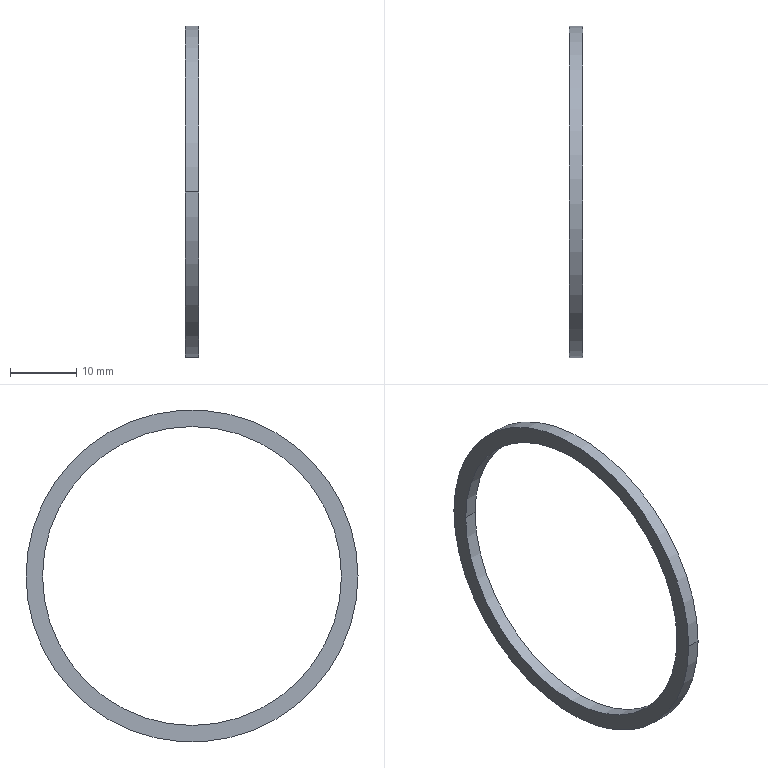Part | NX | features BREP 1 | 1 solid | 6 faces | box 2 x 50 x 50 mm | volume 746.128 mm3 | cylinder 4 | plane 2 | commonest cylinder face diameters 45 x2 50 x2
STEP:
#1=CARTESIAN_POINT('',(-606.355,-34.081,-19.965));
#2=VERTEX_POINT('',#1);
#3=CARTESIAN_POINT('',(-606.355,-79.081,-19.965));
#4=VERTEX_POINT('',#3);
#5=CARTESIAN_POINT('',(-606.355,-56.581,-19.965));
#6=DIRECTION('',(-1.,0.,0.));
#7=DIRECTION('',(0.,-1.,0.));
#8=AXIS2_PLACEMENT_3D('',#5,#6,#7);
#9=CIRCLE('',#8,22.5);
#10=EDGE_CURVE('',#2,#4,#9,.T.);
#11=ORIENTED_EDGE('',*,*,#10,.T.);
#12=CARTESIAN_POINT('',(-604.355,-79.081,-19.965));
#13=VERTEX_POINT('',#12);
#14=CARTESIAN_POINT('',(-606.355,-79.081,-19.965));
#15=DIRECTION('',(1.,0.,0.));
#16=VECTOR('',#15,1000.);
#17=LINE('',#14,#16);
#18=EDGE_CURVE('',#4,#13,#17,.T.);
#19=ORIENTED_EDGE('',*,*,#18,.T.);
#20=CARTESIAN_POINT('',(-604.355,-34.081,-19.965));
#21=VERTEX_POINT('',#20);
#22=CARTESIAN_POINT('',(-604.355,-56.581,-19.965));
#23=DIRECTION('',(-1.,0.,0.));
#24=DIRECTION('',(0.,-1.,0.));
#25=AXIS2_PLACEMENT_3D('',#22,#23,#24);
#26=CIRCLE('',#25,22.5);
#27=EDGE_CURVE('',#21,#13,#26,.T.);
#28=ORIENTED_EDGE('',*,*,#27,.F.);
#29=CARTESIAN_POINT('',(-606.355,-34.081,-19.965));
#30=DIRECTION('',(1.,0.,0.));
#31=VECTOR('',#30,1000.);
#32=LINE('',#29,#31);
#33=EDGE_CURVE('',#2,#21,#32,.T.);
#34=ORIENTED_EDGE('',*,*,#33,.F.);
#35=EDGE_LOOP('',(#11,#19,#28,#34));
#36=FACE_BOUND('',#35,.T.);
#37=CARTESIAN_POINT('',(-606.355,-56.581,-19.965));
#38=DIRECTION('',(1.,0.,0.));
#39=DIRECTION('',(0.,1.,0.));
#40=AXIS2_PLACEMENT_3D('',#37,#38,#39);
#41=CYLINDRICAL_SURFACE('',#40,22.5);
#42=ADVANCED_FACE('',(#36),#41,.F.);
#43=CARTESIAN_POINT('',(-606.355,-81.581,-19.965));
#44=VERTEX_POINT('',#43);
#45=CARTESIAN_POINT('',(-606.355,-31.581,-19.965));
#46=VERTEX_POINT('',#45);
#47=CARTESIAN_POINT('',(-606.355,-56.581,-19.965));
#48=DIRECTION('',(-1.,0.,0.));
#49=DIRECTION('',(0.,-1.,0.));
#50=AXIS2_PLACEMENT_3D('',#47,#48,#49);
#51=CIRCLE('',#50,25.);
#52=EDGE_CURVE('',#44,#46,#51,.T.);
#53=ORIENTED_EDGE('',*,*,#52,.F.);
#54=CARTESIAN_POINT('',(-604.355,-81.581,-19.965));
#55=VERTEX_POINT('',#54);
#56=CARTESIAN_POINT('',(-606.355,-81.581,-19.965));
#57=DIRECTION('',(1.,0.,0.));
#58=VECTOR('',#57,1000.);
#59=LINE('',#56,#58);
#60=EDGE_CURVE('',#44,#55,#59,.T.);
#61=ORIENTED_EDGE('',*,*,#60,.T.);
#62=CARTESIAN_POINT('',(-604.355,-31.581,-19.965));
#63=VERTEX_POINT('',#62);
#64=CARTESIAN_POINT('',(-604.355,-56.581,-19.965));
#65=DIRECTION('',(-1.,0.,0.));
#66=DIRECTION('',(0.,-1.,0.));
#67=AXIS2_PLACEMENT_3D('',#64,#65,#66);
#68=CIRCLE('',#67,25.);
#69=EDGE_CURVE('',#55,#63,#68,.T.);
#70=ORIENTED_EDGE('',*,*,#69,.T.);
#71=CARTESIAN_POINT('',(-606.355,-31.581,-19.965));
#72=DIRECTION('',(1.,0.,0.));
#73=VECTOR('',#72,1000.);
#74=LINE('',#71,#73);
#75=EDGE_CURVE('',#46,#63,#74,.T.);
#76=ORIENTED_EDGE('',*,*,#75,.F.);
#77=EDGE_LOOP('',(#53,#61,#70,#76));
#78=FACE_BOUND('',#77,.T.);
#79=CARTESIAN_POINT('',(-606.355,-56.581,-19.965));
#80=DIRECTION('',(1.,0.,0.));
#81=DIRECTION('',(0.,1.,0.));
#82=AXIS2_PLACEMENT_3D('',#79,#80,#81);
#83=CYLINDRICAL_SURFACE('',#82,25.);
#84=ADVANCED_FACE('',(#78),#83,.T.);
#85=CARTESIAN_POINT('',(-606.355,-56.581,-19.965));
#86=DIRECTION('',(-1.,0.,0.));
#87=DIRECTION('',(0.,-1.,0.));
#88=AXIS2_PLACEMENT_3D('',#85,#86,#87);
#89=CIRCLE('',#88,25.);
#90=EDGE_CURVE('',#46,#44,#89,.T.);
#91=ORIENTED_EDGE('',*,*,#90,.T.);
#92=ORIENTED_EDGE('',*,*,#52,.T.);
#93=EDGE_LOOP('',(#91,#92));
#94=FACE_BOUND('',#93,.T.);
#95=ORIENTED_EDGE('',*,*,#10,.F.);
#96=CARTESIAN_POINT('',(-606.355,-56.581,-19.965));
#97=DIRECTION('',(-1.,0.,0.));
#98=DIRECTION('',(0.,-1.,0.));
#99=AXIS2_PLACEMENT_3D('',#96,#97,#98);
#100=CIRCLE('',#99,22.5);
#101=EDGE_CURVE('',#4,#2,#100,.T.);
#102=ORIENTED_EDGE('',*,*,#101,.F.);
#103=EDGE_LOOP('',(#95,#102));
#104=FACE_BOUND('',#103,.T.);
#105=CARTESIAN_POINT('',(-606.355,-56.581,-19.965));
#106=DIRECTION('',(-1.,0.,0.));
#107=DIRECTION('',(0.,-1.,0.));
#108=AXIS2_PLACEMENT_3D('',#105,#106,#107);
#109=PLANE('',#108);
#110=ADVANCED_FACE('',(#94,#104),#109,.T.);
#111=CARTESIAN_POINT('',(-604.355,-56.581,-19.965));
#112=DIRECTION('',(-1.,0.,0.));
#113=DIRECTION('',(0.,-1.,0.));
#114=AXIS2_PLACEMENT_3D('',#111,#112,#113);
#115=CIRCLE('',#114,25.);
#116=EDGE_CURVE('',#63,#55,#115,.T.);
#117=ORIENTED_EDGE('',*,*,#116,.F.);
#118=ORIENTED_EDGE('',*,*,#69,.F.);
#119=EDGE_LOOP('',(#117,#118));
#120=FACE_BOUND('',#119,.T.);
#121=ORIENTED_EDGE('',*,*,#27,.T.);
#122=CARTESIAN_POINT('',(-604.355,-56.581,-19.965));
#123=DIRECTION('',(-1.,0.,0.));
#124=DIRECTION('',(0.,-1.,0.));
#125=AXIS2_PLACEMENT_3D('',#122,#123,#124);
#126=CIRCLE('',#125,22.5);
#127=EDGE_CURVE('',#13,#21,#126,.T.);
#128=ORIENTED_EDGE('',*,*,#127,.T.);
#129=EDGE_LOOP('',(#121,#128));
#130=FACE_BOUND('',#129,.T.);
#131=CARTESIAN_POINT('',(-604.355,-56.581,-19.965));
#132=DIRECTION('',(-1.,0.,0.));
#133=DIRECTION('',(0.,-1.,0.));
#134=AXIS2_PLACEMENT_3D('',#131,#132,#133);
#135=PLANE('',#134);
#136=ADVANCED_FACE('',(#120,#130),#135,.F.);
#137=ORIENTED_EDGE('',*,*,#60,.F.);
#138=ORIENTED_EDGE('',*,*,#90,.F.);
#139=ORIENTED_EDGE('',*,*,#75,.T.);
#140=ORIENTED_EDGE('',*,*,#116,.T.);
#141=EDGE_LOOP('',(#137,#138,#139,#140));
#142=FACE_BOUND('',#141,.T.);
#143=CARTESIAN_POINT('',(-606.355,-56.581,-19.965));
#144=DIRECTION('',(1.,0.,0.));
#145=DIRECTION('',(0.,1.,0.));
#146=AXIS2_PLACEMENT_3D('',#143,#144,#145);
#147=CYLINDRICAL_SURFACE('',#146,25.);
#148=ADVANCED_FACE('',(#142),#147,.T.);
#149=ORIENTED_EDGE('',*,*,#18,.F.);
#150=ORIENTED_EDGE('',*,*,#101,.T.);
#151=ORIENTED_EDGE('',*,*,#33,.T.);
#152=ORIENTED_EDGE('',*,*,#127,.F.);
#153=EDGE_LOOP('',(#149,#150,#151,#152));
#154=FACE_BOUND('',#153,.T.);
#155=CARTESIAN_POINT('',(-606.355,-56.581,-19.965));
#156=DIRECTION('',(1.,0.,0.));
#157=DIRECTION('',(0.,1.,0.));
#158=AXIS2_PLACEMENT_3D('',#155,#156,#157);
#159=CYLINDRICAL_SURFACE('',#158,22.5);
#160=ADVANCED_FACE('',(#154),#159,.F.);
#161=CLOSED_SHELL('',(#42,#84,#110,#136,#148,#160));
#162=MANIFOLD_SOLID_BREP('',#161);
#163=(LENGTH_UNIT()NAMED_UNIT(*)SI_UNIT(.MILLI.,.METRE.));
#164=UNCERTAINTY_MEASURE_WITH_UNIT(LENGTH_MEASURE(0.00001),#163,'','');
#165=(NAMED_UNIT(*)PLANE_ANGLE_UNIT()SI_UNIT($,.RADIAN.));
#166=(NAMED_UNIT(*)SI_UNIT($,.STERADIAN.)SOLID_ANGLE_UNIT());
#167=(GEOMETRIC_REPRESENTATION_CONTEXT(3)GLOBAL_UNCERTAINTY_ASSIGNED_CONTEXT((#164))GLOBAL_UNIT_ASSIGNED_CONTEXT((#163,#165,#166))REPRESENTATION_CONTEXT('',''));
#168=ADVANCED_BREP_SHAPE_REPRESENTATION('',(#162),#167);